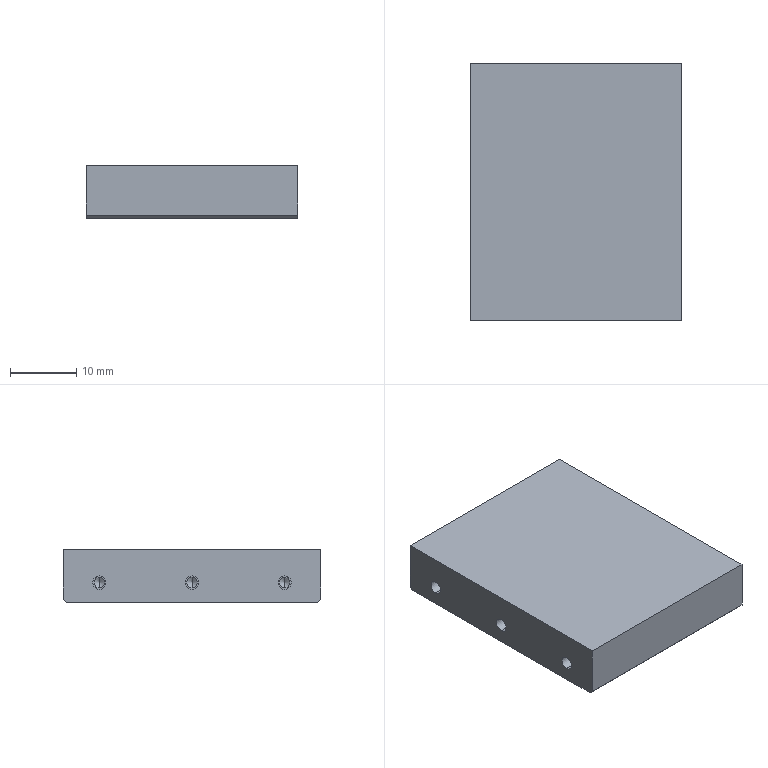Part | STEP file | ASND-0110-OPT-CO40-X-V1.0.5 mounting plate | 1 solid | 78 faces | box 32 x 39 x 8 mm | volume 9600 mm3 | cylinder 40 | cone 20 | plane 18 | commonest cylinder face diameters 1.6 x12 2 x12 3.3 x8 4 x8